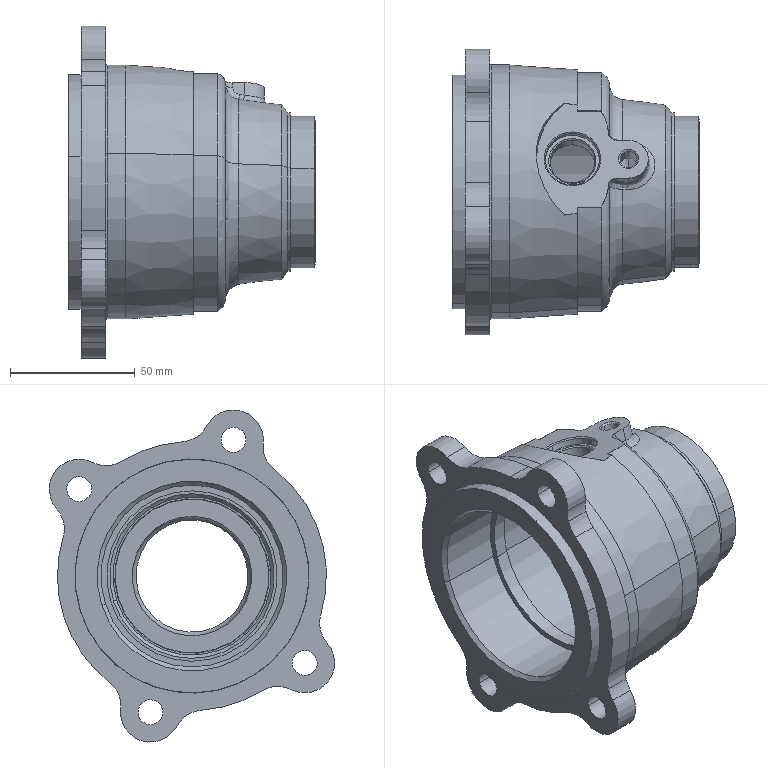Part | NX | features BREP 1 | 1 solid | 140 faces | box 99.1 x 114.53 x 133.325 mm | volume 312332 mm3 | cylinder 65 | plane 23 | cone 22 | torus 18 | spline 12 | commonest cylinder face diameters 24 x16 10 x8 108 x5 96 x3 6.8 x2 18 x2